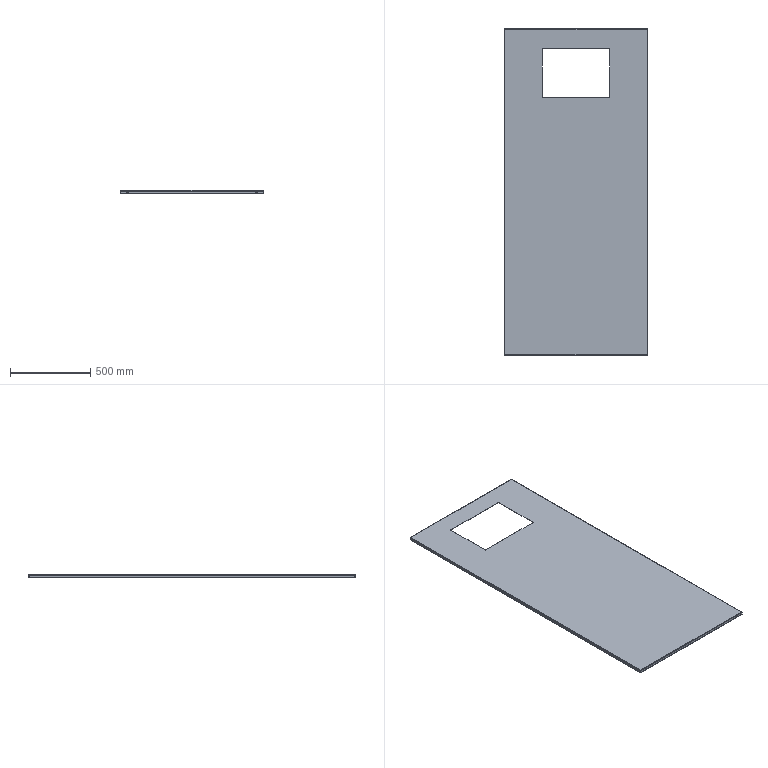Part | STEP file | 750078411 | 1 solid | 70 faces | box 896 x 2036 x 20 mm | volume 3760897 mm3 | plane 50 | cylinder 20 | commonest cylinder face diameters 2 x4 4 x4 6 x4 8 x4 9 x4